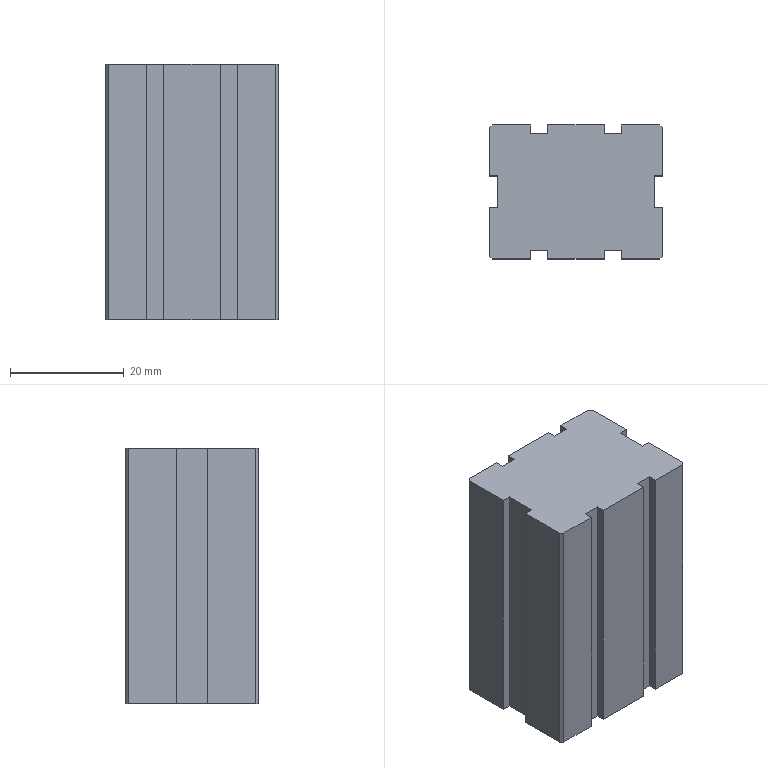Part | SolidWorks | features Extrusion 1 | 1 solid | 34 faces | box 30.5 x 23.5 x 45 mm | volume 30669 mm3 | plane 34
STEP:
#1=CARTESIAN_POINT('',(-8.,11.75,0.));
#2=VERTEX_POINT('',#1);
#3=CARTESIAN_POINT('',(-14.75,11.75,0.));
#4=VERTEX_POINT('',#3);
#5=CARTESIAN_POINT('',(-14.75,11.75,0.));
#6=DIRECTION('',(-1.,0.,0.));
#7=VECTOR('',#6,1000.);
#8=LINE('',#5,#7);
#9=EDGE_CURVE('',#2,#4,#8,.T.);
#10=ORIENTED_EDGE('',*,*,#9,.T.);
#11=CARTESIAN_POINT('',(-14.75,11.75,45.));
#12=VERTEX_POINT('',#11);
#13=CARTESIAN_POINT('',(-14.75,11.75,45.));
#14=DIRECTION('',(0.,0.,-1.));
#15=VECTOR('',#14,1000.);
#16=LINE('',#13,#15);
#17=EDGE_CURVE('',#12,#4,#16,.T.);
#18=ORIENTED_EDGE('',*,*,#17,.F.);
#19=CARTESIAN_POINT('',(-8.,11.75,45.));
#20=VERTEX_POINT('',#19);
#21=CARTESIAN_POINT('',(-14.75,11.75,45.));
#22=DIRECTION('',(-1.,0.,0.));
#23=VECTOR('',#22,1000.);
#24=LINE('',#21,#23);
#25=EDGE_CURVE('',#20,#12,#24,.T.);
#26=ORIENTED_EDGE('',*,*,#25,.F.);
#27=CARTESIAN_POINT('',(-8.,11.75,45.));
#28=DIRECTION('',(0.,0.,-1.));
#29=VECTOR('',#28,1000.);
#30=LINE('',#27,#29);
#31=EDGE_CURVE('',#20,#2,#30,.T.);
#32=ORIENTED_EDGE('',*,*,#31,.T.);
#33=EDGE_LOOP('',(#10,#18,#26,#32));
#34=FACE_OUTER_BOUND('',#33,.T.);
#35=CARTESIAN_POINT('',(-14.75,11.75,45.));
#36=DIRECTION('',(0.,-1.,0.));
#37=DIRECTION('',(1.,0.,0.));
#38=AXIS2_PLACEMENT_3D('',#35,#36,#37);
#39=PLANE('',#38);
#40=ADVANCED_FACE('',(#34),#39,.F.);
#41=CARTESIAN_POINT('',(-15.25,11.25,0.));
#42=VERTEX_POINT('',#41);
#43=CARTESIAN_POINT('',(-15.25,11.25,0.));
#44=DIRECTION('',(-0.7071,-0.7071,0.));
#45=VECTOR('',#44,1000.);
#46=LINE('',#43,#45);
#47=EDGE_CURVE('',#4,#42,#46,.T.);
#48=ORIENTED_EDGE('',*,*,#47,.T.);
#49=CARTESIAN_POINT('',(-15.25,11.25,45.));
#50=VERTEX_POINT('',#49);
#51=CARTESIAN_POINT('',(-15.25,11.25,45.));
#52=DIRECTION('',(0.,0.,-1.));
#53=VECTOR('',#52,1000.);
#54=LINE('',#51,#53);
#55=EDGE_CURVE('',#50,#42,#54,.T.);
#56=ORIENTED_EDGE('',*,*,#55,.F.);
#57=CARTESIAN_POINT('',(-15.25,11.25,45.));
#58=DIRECTION('',(-0.7071,-0.7071,0.));
#59=VECTOR('',#58,1000.);
#60=LINE('',#57,#59);
#61=EDGE_CURVE('',#12,#50,#60,.T.);
#62=ORIENTED_EDGE('',*,*,#61,.F.);
#63=ORIENTED_EDGE('',*,*,#17,.T.);
#64=EDGE_LOOP('',(#48,#56,#62,#63));
#65=FACE_OUTER_BOUND('',#64,.T.);
#66=CARTESIAN_POINT('',(-15.25,11.25,45.));
#67=DIRECTION('',(0.7071,-0.7071,0.));
#68=DIRECTION('',(0.7071,0.7071,0.));
#69=AXIS2_PLACEMENT_3D('',#66,#67,#68);
#70=PLANE('',#69);
#71=ADVANCED_FACE('',(#65),#70,.F.);
#72=CARTESIAN_POINT('',(-15.25,2.786,0.));
#73=VERTEX_POINT('',#72);
#74=CARTESIAN_POINT('',(-15.25,11.25,0.));
#75=DIRECTION('',(0.,-1.,0.));
#76=VECTOR('',#75,1000.);
#77=LINE('',#74,#76);
#78=EDGE_CURVE('',#42,#73,#77,.T.);
#79=ORIENTED_EDGE('',*,*,#78,.T.);
#80=CARTESIAN_POINT('',(-15.25,2.786,45.));
#81=VERTEX_POINT('',#80);
#82=CARTESIAN_POINT('',(-15.25,2.786,45.));
#83=DIRECTION('',(0.,0.,-1.));
#84=VECTOR('',#83,1000.);
#85=LINE('',#82,#84);
#86=EDGE_CURVE('',#81,#73,#85,.T.);
#87=ORIENTED_EDGE('',*,*,#86,.F.);
#88=CARTESIAN_POINT('',(-15.25,11.25,45.));
#89=DIRECTION('',(0.,-1.,0.));
#90=VECTOR('',#89,1000.);
#91=LINE('',#88,#90);
#92=EDGE_CURVE('',#50,#81,#91,.T.);
#93=ORIENTED_EDGE('',*,*,#92,.F.);
#94=ORIENTED_EDGE('',*,*,#55,.T.);
#95=EDGE_LOOP('',(#79,#87,#93,#94));
#96=FACE_OUTER_BOUND('',#95,.T.);
#97=CARTESIAN_POINT('',(-15.25,11.25,45.));
#98=DIRECTION('',(1.,0.,0.));
#99=DIRECTION('',(0.,0.,-1.));
#100=AXIS2_PLACEMENT_3D('',#97,#98,#99);
#101=PLANE('',#100);
#102=ADVANCED_FACE('',(#96),#101,.F.);
#103=CARTESIAN_POINT('',(-13.75,2.786,0.));
#104=VERTEX_POINT('',#103);
#105=CARTESIAN_POINT('',(-15.25,2.786,0.));
#106=DIRECTION('',(1.,0.,0.));
#107=VECTOR('',#106,1000.);
#108=LINE('',#105,#107);
#109=EDGE_CURVE('',#73,#104,#108,.T.);
#110=ORIENTED_EDGE('',*,*,#109,.T.);
#111=CARTESIAN_POINT('',(-13.75,2.786,45.));
#112=VERTEX_POINT('',#111);
#113=CARTESIAN_POINT('',(-13.75,2.786,45.));
#114=DIRECTION('',(0.,0.,-1.));
#115=VECTOR('',#114,1000.);
#116=LINE('',#113,#115);
#117=EDGE_CURVE('',#112,#104,#116,.T.);
#118=ORIENTED_EDGE('',*,*,#117,.F.);
#119=CARTESIAN_POINT('',(-15.25,2.786,45.));
#120=DIRECTION('',(1.,0.,0.));
#121=VECTOR('',#120,1000.);
#122=LINE('',#119,#121);
#123=EDGE_CURVE('',#81,#112,#122,.T.);
#124=ORIENTED_EDGE('',*,*,#123,.F.);
#125=ORIENTED_EDGE('',*,*,#86,.T.);
#126=EDGE_LOOP('',(#110,#118,#124,#125));
#127=FACE_OUTER_BOUND('',#126,.T.);
#128=CARTESIAN_POINT('',(-15.25,2.786,45.));
#129=DIRECTION('',(0.,1.,0.));
#130=DIRECTION('',(0.,0.,1.));
#131=AXIS2_PLACEMENT_3D('',#128,#129,#130);
#132=PLANE('',#131);
#133=ADVANCED_FACE('',(#127),#132,.F.);
#134=CARTESIAN_POINT('',(-13.75,-2.786,0.));
#135=VERTEX_POINT('',#134);
#136=CARTESIAN_POINT('',(-13.75,2.786,0.));
#137=DIRECTION('',(0.,-1.,0.));
#138=VECTOR('',#137,1000.);
#139=LINE('',#136,#138);
#140=EDGE_CURVE('',#104,#135,#139,.T.);
#141=ORIENTED_EDGE('',*,*,#140,.T.);
#142=CARTESIAN_POINT('',(-13.75,-2.786,45.));
#143=VERTEX_POINT('',#142);
#144=CARTESIAN_POINT('',(-13.75,-2.786,45.));
#145=DIRECTION('',(0.,0.,-1.));
#146=VECTOR('',#145,1000.);
#147=LINE('',#144,#146);
#148=EDGE_CURVE('',#143,#135,#147,.T.);
#149=ORIENTED_EDGE('',*,*,#148,.F.);
#150=CARTESIAN_POINT('',(-13.75,2.786,45.));
#151=DIRECTION('',(0.,-1.,0.));
#152=VECTOR('',#151,1000.);
#153=LINE('',#150,#152);
#154=EDGE_CURVE('',#112,#143,#153,.T.);
#155=ORIENTED_EDGE('',*,*,#154,.F.);
#156=ORIENTED_EDGE('',*,*,#117,.T.);
#157=EDGE_LOOP('',(#141,#149,#155,#156));
#158=FACE_OUTER_BOUND('',#157,.T.);
#159=CARTESIAN_POINT('',(-13.75,2.786,45.));
#160=DIRECTION('',(1.,0.,0.));
#161=DIRECTION('',(0.,0.,-1.));
#162=AXIS2_PLACEMENT_3D('',#159,#160,#161);
#163=PLANE('',#162);
#164=ADVANCED_FACE('',(#158),#163,.F.);
#165=CARTESIAN_POINT('',(-15.25,-2.786,0.));
#166=VERTEX_POINT('',#165);
#167=CARTESIAN_POINT('',(-15.25,-2.786,0.));
#168=DIRECTION('',(-1.,0.,0.));
#169=VECTOR('',#168,1000.);
#170=LINE('',#167,#169);
#171=EDGE_CURVE('',#135,#166,#170,.T.);
#172=ORIENTED_EDGE('',*,*,#171,.T.);
#173=CARTESIAN_POINT('',(-15.25,-2.786,45.));
#174=VERTEX_POINT('',#173);
#175=CARTESIAN_POINT('',(-15.25,-2.786,45.));
#176=DIRECTION('',(0.,0.,-1.));
#177=VECTOR('',#176,1000.);
#178=LINE('',#175,#177);
#179=EDGE_CURVE('',#174,#166,#178,.T.);
#180=ORIENTED_EDGE('',*,*,#179,.F.);
#181=CARTESIAN_POINT('',(-15.25,-2.786,45.));
#182=DIRECTION('',(-1.,0.,0.));
#183=VECTOR('',#182,1000.);
#184=LINE('',#181,#183);
#185=EDGE_CURVE('',#143,#174,#184,.T.);
#186=ORIENTED_EDGE('',*,*,#185,.F.);
#187=ORIENTED_EDGE('',*,*,#148,.T.);
#188=EDGE_LOOP('',(#172,#180,#186,#187));
#189=FACE_OUTER_BOUND('',#188,.T.);
#190=CARTESIAN_POINT('',(-15.25,-2.786,45.));
#191=DIRECTION('',(0.,-1.,0.));
#192=DIRECTION('',(0.,0.,-1.));
#193=AXIS2_PLACEMENT_3D('',#190,#191,#192);
#194=PLANE('',#193);
#195=ADVANCED_FACE('',(#189),#194,.F.);
#196=CARTESIAN_POINT('',(-15.25,-11.25,0.));
#197=VERTEX_POINT('',#196);
#198=CARTESIAN_POINT('',(-15.25,-2.786,0.));
#199=DIRECTION('',(0.,-1.,0.));
#200=VECTOR('',#199,1000.);
#201=LINE('',#198,#200);
#202=EDGE_CURVE('',#166,#197,#201,.T.);
#203=ORIENTED_EDGE('',*,*,#202,.T.);
#204=CARTESIAN_POINT('',(-15.25,-11.25,45.));
#205=VERTEX_POINT('',#204);
#206=CARTESIAN_POINT('',(-15.25,-11.25,45.));
#207=DIRECTION('',(0.,0.,-1.));
#208=VECTOR('',#207,1000.);
#209=LINE('',#206,#208);
#210=EDGE_CURVE('',#205,#197,#209,.T.);
#211=ORIENTED_EDGE('',*,*,#210,.F.);
#212=CARTESIAN_POINT('',(-15.25,-2.786,45.));
#213=DIRECTION('',(0.,-1.,0.));
#214=VECTOR('',#213,1000.);
#215=LINE('',#212,#214);
#216=EDGE_CURVE('',#174,#205,#215,.T.);
#217=ORIENTED_EDGE('',*,*,#216,.F.);
#218=ORIENTED_EDGE('',*,*,#179,.T.);
#219=EDGE_LOOP('',(#203,#211,#217,#218));
#220=FACE_OUTER_BOUND('',#219,.T.);
#221=CARTESIAN_POINT('',(-15.25,-2.786,45.));
#222=DIRECTION('',(1.,0.,0.));
#223=DIRECTION('',(0.,1.,0.));
#224=AXIS2_PLACEMENT_3D('',#221,#222,#223);
#225=PLANE('',#224);
#226=ADVANCED_FACE('',(#220),#225,.F.);
#227=CARTESIAN_POINT('',(-14.75,-11.75,0.));
#228=VERTEX_POINT('',#227);
#229=CARTESIAN_POINT('',(-15.25,-11.25,0.));
#230=DIRECTION('',(0.7071,-0.7071,0.));
#231=VECTOR('',#230,1000.);
#232=LINE('',#229,#231);
#233=EDGE_CURVE('',#197,#228,#232,.T.);
#234=ORIENTED_EDGE('',*,*,#233,.T.);
#235=CARTESIAN_POINT('',(-14.75,-11.75,45.));
#236=VERTEX_POINT('',#235);
#237=CARTESIAN_POINT('',(-14.75,-11.75,45.));
#238=DIRECTION('',(0.,0.,-1.));
#239=VECTOR('',#238,1000.);
#240=LINE('',#237,#239);
#241=EDGE_CURVE('',#236,#228,#240,.T.);
#242=ORIENTED_EDGE('',*,*,#241,.F.);
#243=CARTESIAN_POINT('',(-15.25,-11.25,45.));
#244=DIRECTION('',(0.7071,-0.7071,0.));
#245=VECTOR('',#244,1000.);
#246=LINE('',#243,#245);
#247=EDGE_CURVE('',#205,#236,#246,.T.);
#248=ORIENTED_EDGE('',*,*,#247,.F.);
#249=ORIENTED_EDGE('',*,*,#210,.T.);
#250=EDGE_LOOP('',(#234,#242,#248,#249));
#251=FACE_OUTER_BOUND('',#250,.T.);
#252=CARTESIAN_POINT('',(-15.25,-11.25,45.));
#253=DIRECTION('',(0.7071,0.7071,0.));
#254=DIRECTION('',(-0.7071,0.7071,0.));
#255=AXIS2_PLACEMENT_3D('',#252,#253,#254);
#256=PLANE('',#255);
#257=ADVANCED_FACE('',(#251),#256,.F.);
#258=CARTESIAN_POINT('',(-8.,-11.75,0.));
#259=VERTEX_POINT('',#258);
#260=CARTESIAN_POINT('',(-14.75,-11.75,0.));
#261=DIRECTION('',(1.,0.,0.));
#262=VECTOR('',#261,1000.);
#263=LINE('',#260,#262);
#264=EDGE_CURVE('',#228,#259,#263,.T.);
#265=ORIENTED_EDGE('',*,*,#264,.T.);
#266=CARTESIAN_POINT('',(-8.,-11.75,45.));
#267=VERTEX_POINT('',#266);
#268=CARTESIAN_POINT('',(-8.,-11.75,45.));
#269=DIRECTION('',(0.,0.,-1.));
#270=VECTOR('',#269,1000.);
#271=LINE('',#268,#270);
#272=EDGE_CURVE('',#267,#259,#271,.T.);
#273=ORIENTED_EDGE('',*,*,#272,.F.);
#274=CARTESIAN_POINT('',(-14.75,-11.75,45.));
#275=DIRECTION('',(1.,0.,0.));
#276=VECTOR('',#275,1000.);
#277=LINE('',#274,#276);
#278=EDGE_CURVE('',#236,#267,#277,.T.);
#279=ORIENTED_EDGE('',*,*,#278,.F.);
#280=ORIENTED_EDGE('',*,*,#241,.T.);
#281=EDGE_LOOP('',(#265,#273,#279,#280));
#282=FACE_OUTER_BOUND('',#281,.T.);
#283=CARTESIAN_POINT('',(-14.75,-11.75,45.));
#284=DIRECTION('',(0.,1.,0.));
#285=DIRECTION('',(0.,0.,1.));
#286=AXIS2_PLACEMENT_3D('',#283,#284,#285);
#287=PLANE('',#286);
#288=ADVANCED_FACE('',(#282),#287,.F.);
#289=CARTESIAN_POINT('',(-8.,-10.25,0.));
#290=VERTEX_POINT('',#289);
#291=CARTESIAN_POINT('',(-8.,-11.75,0.));
#292=DIRECTION('',(0.,1.,0.));
#293=VECTOR('',#292,1000.);
#294=LINE('',#291,#293);
#295=EDGE_CURVE('',#259,#290,#294,.T.);
#296=ORIENTED_EDGE('',*,*,#295,.T.);
#297=CARTESIAN_POINT('',(-8.,-10.25,45.));
#298=VERTEX_POINT('',#297);
#299=CARTESIAN_POINT('',(-8.,-10.25,45.));
#300=DIRECTION('',(0.,0.,-1.));
#301=VECTOR('',#300,1000.);
#302=LINE('',#299,#301);
#303=EDGE_CURVE('',#298,#290,#302,.T.);
#304=ORIENTED_EDGE('',*,*,#303,.F.);
#305=CARTESIAN_POINT('',(-8.,-11.75,45.));
#306=DIRECTION('',(0.,1.,0.));
#307=VECTOR('',#306,1000.);
#308=LINE('',#305,#307);
#309=EDGE_CURVE('',#267,#298,#308,.T.);
#310=ORIENTED_EDGE('',*,*,#309,.F.);
#311=ORIENTED_EDGE('',*,*,#272,.T.);
#312=EDGE_LOOP('',(#296,#304,#310,#311));
#313=FACE_OUTER_BOUND('',#312,.T.);
#314=CARTESIAN_POINT('',(-8.,-11.75,45.));
#315=DIRECTION('',(-1.,0.,0.));
#316=DIRECTION('',(0.,0.,1.));
#317=AXIS2_PLACEMENT_3D('',#314,#315,#316);
#318=PLANE('',#317);
#319=ADVANCED_FACE('',(#313),#318,.F.);
#320=CARTESIAN_POINT('',(-5.,-10.25,0.));
#321=VERTEX_POINT('',#320);
#322=CARTESIAN_POINT('',(-8.,-10.25,0.));
#323=DIRECTION('',(1.,0.,0.));
#324=VECTOR('',#323,1000.);
#325=LINE('',#322,#324);
#326=EDGE_CURVE('',#290,#321,#325,.T.);
#327=ORIENTED_EDGE('',*,*,#326,.T.);
#328=CARTESIAN_POINT('',(-5.,-10.25,45.));
#329=VERTEX_POINT('',#328);
#330=CARTESIAN_POINT('',(-5.,-10.25,45.));
#331=DIRECTION('',(0.,0.,-1.));
#332=VECTOR('',#331,1000.);
#333=LINE('',#330,#332);
#334=EDGE_CURVE('',#329,#321,#333,.T.);
#335=ORIENTED_EDGE('',*,*,#334,.F.);
#336=CARTESIAN_POINT('',(-8.,-10.25,45.));
#337=DIRECTION('',(1.,0.,0.));
#338=VECTOR('',#337,1000.);
#339=LINE('',#336,#338);
#340=EDGE_CURVE('',#298,#329,#339,.T.);
#341=ORIENTED_EDGE('',*,*,#340,.F.);
#342=ORIENTED_EDGE('',*,*,#303,.T.);
#343=EDGE_LOOP('',(#327,#335,#341,#342));
#344=FACE_OUTER_BOUND('',#343,.T.);
#345=CARTESIAN_POINT('',(-8.,-10.25,45.));
#346=DIRECTION('',(0.,1.,0.));
#347=DIRECTION('',(0.,0.,1.));
#348=AXIS2_PLACEMENT_3D('',#345,#346,#347);
#349=PLANE('',#348);
#350=ADVANCED_FACE('',(#344),#349,.F.);
#351=CARTESIAN_POINT('',(-5.,-11.75,0.));
#352=VERTEX_POINT('',#351);
#353=CARTESIAN_POINT('',(-5.,-10.25,0.));
#354=DIRECTION('',(0.,-1.,0.));
#355=VECTOR('',#354,1000.);
#356=LINE('',#353,#355);
#357=EDGE_CURVE('',#321,#352,#356,.T.);
#358=ORIENTED_EDGE('',*,*,#357,.T.);
#359=CARTESIAN_POINT('',(-5.,-11.75,45.));
#360=VERTEX_POINT('',#359);
#361=CARTESIAN_POINT('',(-5.,-11.75,45.));
#362=DIRECTION('',(0.,0.,-1.));
#363=VECTOR('',#362,1000.);
#364=LINE('',#361,#363);
#365=EDGE_CURVE('',#360,#352,#364,.T.);
#366=ORIENTED_EDGE('',*,*,#365,.F.);
#367=CARTESIAN_POINT('',(-5.,-10.25,45.));
#368=DIRECTION('',(0.,-1.,0.));
#369=VECTOR('',#368,1000.);
#370=LINE('',#367,#369);
#371=EDGE_CURVE('',#329,#360,#370,.T.);
#372=ORIENTED_EDGE('',*,*,#371,.F.);
#373=ORIENTED_EDGE('',*,*,#334,.T.);
#374=EDGE_LOOP('',(#358,#366,#372,#373));
#375=FACE_OUTER_BOUND('',#374,.T.);
#376=CARTESIAN_POINT('',(-5.,-10.25,45.));
#377=DIRECTION('',(1.,0.,0.));
#378=DIRECTION('',(0.,0.,-1.));
#379=AXIS2_PLACEMENT_3D('',#376,#377,#378);
#380=PLANE('',#379);
#381=ADVANCED_FACE('',(#375),#380,.F.);
#382=CARTESIAN_POINT('',(5.,-11.75,0.));
#383=VERTEX_POINT('',#382);
#384=CARTESIAN_POINT('',(-5.,-11.75,0.));
#385=DIRECTION('',(1.,0.,0.));
#386=VECTOR('',#385,1000.);
#387=LINE('',#384,#386);
#388=EDGE_CURVE('',#352,#383,#387,.T.);
#389=ORIENTED_EDGE('',*,*,#388,.T.);
#390=CARTESIAN_POINT('',(5.,-11.75,45.));
#391=VERTEX_POINT('',#390);
#392=CARTESIAN_POINT('',(5.,-11.75,45.));
#393=DIRECTION('',(0.,0.,-1.));
#394=VECTOR('',#393,1000.);
#395=LINE('',#392,#394);
#396=EDGE_CURVE('',#391,#383,#395,.T.);
#397=ORIENTED_EDGE('',*,*,#396,.F.);
#398=CARTESIAN_POINT('',(-5.,-11.75,45.));
#399=DIRECTION('',(1.,0.,0.));
#400=VECTOR('',#399,1000.);
#401=LINE('',#398,#400);
#402=EDGE_CURVE('',#360,#391,#401,.T.);
#403=ORIENTED_EDGE('',*,*,#402,.F.);
#404=ORIENTED_EDGE('',*,*,#365,.T.);
#405=EDGE_LOOP('',(#389,#397,#403,#404));
#406=FACE_OUTER_BOUND('',#405,.T.);
#407=CARTESIAN_POINT('',(-5.,-11.75,45.));
#408=DIRECTION('',(0.,1.,0.));
#409=DIRECTION('',(0.,0.,1.));
#410=AXIS2_PLACEMENT_3D('',#407,#408,#409);
#411=PLANE('',#410);
#412=ADVANCED_FACE('',(#406),#411,.F.);
#413=CARTESIAN_POINT('',(5.,-10.25,0.));
#414=VERTEX_POINT('',#413);
#415=CARTESIAN_POINT('',(5.,-10.25,0.));
#416=DIRECTION('',(0.,1.,0.));
#417=VECTOR('',#416,1000.);
#418=LINE('',#415,#417);
#419=EDGE_CURVE('',#383,#414,#418,.T.);
#420=ORIENTED_EDGE('',*,*,#419,.T.);
#421=CARTESIAN_POINT('',(5.,-10.25,45.));
#422=VERTEX_POINT('',#421);
#423=CARTESIAN_POINT('',(5.,-10.25,45.));
#424=DIRECTION('',(0.,0.,-1.));
#425=VECTOR('',#424,1000.);
#426=LINE('',#423,#425);
#427=EDGE_CURVE('',#422,#414,#426,.T.);
#428=ORIENTED_EDGE('',*,*,#427,.F.);
#429=CARTESIAN_POINT('',(5.,-10.25,45.));
#430=DIRECTION('',(0.,1.,0.));
#431=VECTOR('',#430,1000.);
#432=LINE('',#429,#431);
#433=EDGE_CURVE('',#391,#422,#432,.T.);
#434=ORIENTED_EDGE('',*,*,#433,.F.);
#435=ORIENTED_EDGE('',*,*,#396,.T.);
#436=EDGE_LOOP('',(#420,#428,#434,#435));
#437=FACE_OUTER_BOUND('',#436,.T.);
#438=CARTESIAN_POINT('',(5.,-10.25,45.));
#439=DIRECTION('',(-1.,0.,0.));
#440=DIRECTION('',(0.,0.,1.));
#441=AXIS2_PLACEMENT_3D('',#438,#439,#440);
#442=PLANE('',#441);
#443=ADVANCED_FACE('',(#437),#442,.F.);
#444=CARTESIAN_POINT('',(8.,-10.25,0.));
#445=VERTEX_POINT('',#444);
#446=CARTESIAN_POINT('',(8.,-10.25,0.));
#447=DIRECTION('',(1.,0.,0.));
#448=VECTOR('',#447,1000.);
#449=LINE('',#446,#448);
#450=EDGE_CURVE('',#414,#445,#449,.T.);
#451=ORIENTED_EDGE('',*,*,#450,.T.);
#452=CARTESIAN_POINT('',(8.,-10.25,45.));
#453=VERTEX_POINT('',#452);
#454=CARTESIAN_POINT('',(8.,-10.25,45.));
#455=DIRECTION('',(0.,0.,-1.));
#456=VECTOR('',#455,1000.);
#457=LINE('',#454,#456);
#458=EDGE_CURVE('',#453,#445,#457,.T.);
#459=ORIENTED_EDGE('',*,*,#458,.F.);
#460=CARTESIAN_POINT('',(8.,-10.25,45.));
#461=DIRECTION('',(1.,0.,0.));
#462=VECTOR('',#461,1000.);
#463=LINE('',#460,#462);
#464=EDGE_CURVE('',#422,#453,#463,.T.);
#465=ORIENTED_EDGE('',*,*,#464,.F.);
#466=ORIENTED_EDGE('',*,*,#427,.T.);
#467=EDGE_LOOP('',(#451,#459,#465,#466));
#468=FACE_OUTER_BOUND('',#467,.T.);
#469=CARTESIAN_POINT('',(8.,-10.25,45.));
#470=DIRECTION('',(0.,1.,0.));
#471=DIRECTION('',(0.,0.,1.));
#472=AXIS2_PLACEMENT_3D('',#469,#470,#471);
#473=PLANE('',#472);
#474=ADVANCED_FACE('',(#468),#473,.F.);
#475=CARTESIAN_POINT('',(8.,-11.75,0.));
#476=VERTEX_POINT('',#475);
#477=CARTESIAN_POINT('',(8.,-11.75,0.));
#478=DIRECTION('',(0.,-1.,0.));
#479=VECTOR('',#478,1000.);
#480=LINE('',#477,#479);
#481=EDGE_CURVE('',#445,#476,#480,.T.);
#482=ORIENTED_EDGE('',*,*,#481,.T.);
#483=CARTESIAN_POINT('',(8.,-11.75,45.));
#484=VERTEX_POINT('',#483);
#485=CARTESIAN_POINT('',(8.,-11.75,45.));
#486=DIRECTION('',(0.,0.,-1.));
#487=VECTOR('',#486,1000.);
#488=LINE('',#485,#487);
#489=EDGE_CURVE('',#484,#476,#488,.T.);
#490=ORIENTED_EDGE('',*,*,#489,.F.);
#491=CARTESIAN_POINT('',(8.,-11.75,45.));
#492=DIRECTION('',(0.,-1.,0.));
#493=VECTOR('',#492,1000.);
#494=LINE('',#491,#493);
#495=EDGE_CURVE('',#453,#484,#494,.T.);
#496=ORIENTED_EDGE('',*,*,#495,.F.);
#497=ORIENTED_EDGE('',*,*,#458,.T.);
#498=EDGE_LOOP('',(#482,#490,#496,#497));
#499=FACE_OUTER_BOUND('',#498,.T.);
#500=CARTESIAN_POINT('',(8.,-11.75,45.));
#501=DIRECTION('',(1.,0.,0.));
#502=DIRECTION('',(0.,0.,-1.));
#503=AXIS2_PLACEMENT_3D('',#500,#501,#502);
#504=PLANE('',#503);
#505=ADVANCED_FACE('',(#499),#504,.F.);
#506=CARTESIAN_POINT('',(14.75,-11.75,0.));
#507=VERTEX_POINT('',#506);
#508=CARTESIAN_POINT('',(8.,-11.75,0.));
#509=DIRECTION('',(1.,0.,0.));
#510=VECTOR('',#509,1000.);
#511=LINE('',#508,#510);
#512=EDGE_CURVE('',#476,#507,#511,.T.);
#513=ORIENTED_EDGE('',*,*,#512,.T.);
#514=CARTESIAN_POINT('',(14.75,-11.75,45.));
#515=VERTEX_POINT('',#514);
#516=CARTESIAN_POINT('',(14.75,-11.75,45.));
#517=DIRECTION('',(0.,0.,-1.));
#518=VECTOR('',#517,1000.);
#519=LINE('',#516,#518);
#520=EDGE_CURVE('',#515,#507,#519,.T.);
#521=ORIENTED_EDGE('',*,*,#520,.F.);
#522=CARTESIAN_POINT('',(8.,-11.75,45.));
#523=DIRECTION('',(1.,0.,0.));
#524=VECTOR('',#523,1000.);
#525=LINE('',#522,#524);
#526=EDGE_CURVE('',#484,#515,#525,.T.);
#527=ORIENTED_EDGE('',*,*,#526,.F.);
#528=ORIENTED_EDGE('',*,*,#489,.T.);
#529=EDGE_LOOP('',(#513,#521,#527,#528));
#530=FACE_OUTER_BOUND('',#529,.T.);
#531=CARTESIAN_POINT('',(8.,-11.75,45.));
#532=DIRECTION('',(0.,1.,0.));
#533=DIRECTION('',(0.,0.,1.));
#534=AXIS2_PLACEMENT_3D('',#531,#532,#533);
#535=PLANE('',#534);
#536=ADVANCED_FACE('',(#530),#535,.F.);
#537=CARTESIAN_POINT('',(15.25,-11.25,0.));
#538=VERTEX_POINT('',#537);
#539=CARTESIAN_POINT('',(14.75,-11.75,0.));
#540=DIRECTION('',(0.7071,0.7071,0.));
#541=VECTOR('',#540,1000.);
#542=LINE('',#539,#541);
#543=EDGE_CURVE('',#507,#538,#542,.T.);
#544=ORIENTED_EDGE('',*,*,#543,.T.);
#545=CARTESIAN_POINT('',(15.25,-11.25,45.));
#546=VERTEX_POINT('',#545);
#547=CARTESIAN_POINT('',(15.25,-11.25,45.));
#548=DIRECTION('',(0.,0.,-1.));
#549=VECTOR('',#548,1000.);
#550=LINE('',#547,#549);
#551=EDGE_CURVE('',#546,#538,#550,.T.);
#552=ORIENTED_EDGE('',*,*,#551,.F.);
#553=CARTESIAN_POINT('',(14.75,-11.75,45.));
#554=DIRECTION('',(0.7071,0.7071,0.));
#555=VECTOR('',#554,1000.);
#556=LINE('',#553,#555);
#557=EDGE_CURVE('',#515,#546,#556,.T.);
#558=ORIENTED_EDGE('',*,*,#557,.F.);
#559=ORIENTED_EDGE('',*,*,#520,.T.);
#560=EDGE_LOOP('',(#544,#552,#558,#559));
#561=FACE_OUTER_BOUND('',#560,.T.);
#562=CARTESIAN_POINT('',(14.75,-11.75,45.));
#563=DIRECTION('',(-0.7071,0.7071,0.));
#564=DIRECTION('',(-0.7071,-0.7071,0.));
#565=AXIS2_PLACEMENT_3D('',#562,#563,#564);
#566=PLANE('',#565);
#567=ADVANCED_FACE('',(#561),#566,.F.);
#568=CARTESIAN_POINT('',(15.25,-2.786,0.));
#569=VERTEX_POINT('',#568);
#570=CARTESIAN_POINT('',(15.25,-2.786,0.));
#571=DIRECTION('',(0.,1.,0.));
#572=VECTOR('',#571,1000.);
#573=LINE('',#570,#572);
#574=EDGE_CURVE('',#538,#569,#573,.T.);
#575=ORIENTED_EDGE('',*,*,#574,.T.);
#576=CARTESIAN_POINT('',(15.25,-2.786,45.));
#577=VERTEX_POINT('',#576);
#578=CARTESIAN_POINT('',(15.25,-2.786,45.));
#579=DIRECTION('',(0.,0.,-1.));
#580=VECTOR('',#579,1000.);
#581=LINE('',#578,#580);
#582=EDGE_CURVE('',#577,#569,#581,.T.);
#583=ORIENTED_EDGE('',*,*,#582,.F.);
#584=CARTESIAN_POINT('',(15.25,-2.786,45.));
#585=DIRECTION('',(0.,1.,0.));
#586=VECTOR('',#585,1000.);
#587=LINE('',#584,#586);
#588=EDGE_CURVE('',#546,#577,#587,.T.);
#589=ORIENTED_EDGE('',*,*,#588,.F.);
#590=ORIENTED_EDGE('',*,*,#551,.T.);
#591=EDGE_LOOP('',(#575,#583,#589,#590));
#592=FACE_OUTER_BOUND('',#591,.T.);
#593=CARTESIAN_POINT('',(15.25,-2.786,45.));
#594=DIRECTION('',(-1.,0.,0.));
#595=DIRECTION('',(0.,-1.,0.));
#596=AXIS2_PLACEMENT_3D('',#593,#594,#595);
#597=PLANE('',#596);
#598=ADVANCED_FACE('',(#592),#597,.F.);
#599=CARTESIAN_POINT('',(13.75,-2.786,0.));
#600=VERTEX_POINT('',#599);
#601=CARTESIAN_POINT('',(15.25,-2.786,0.));
#602=DIRECTION('',(-1.,0.,0.));
#603=VECTOR('',#602,1000.);
#604=LINE('',#601,#603);
#605=EDGE_CURVE('',#569,#600,#604,.T.);
#606=ORIENTED_EDGE('',*,*,#605,.T.);
#607=CARTESIAN_POINT('',(13.75,-2.786,45.));
#608=VERTEX_POINT('',#607);
#609=CARTESIAN_POINT('',(13.75,-2.786,45.));
#610=DIRECTION('',(0.,0.,-1.));
#611=VECTOR('',#610,1000.);
#612=LINE('',#609,#611);
#613=EDGE_CURVE('',#608,#600,#612,.T.);
#614=ORIENTED_EDGE('',*,*,#613,.F.);
#615=CARTESIAN_POINT('',(15.25,-2.786,45.));
#616=DIRECTION('',(-1.,0.,0.));
#617=VECTOR('',#616,1000.);
#618=LINE('',#615,#617);
#619=EDGE_CURVE('',#577,#608,#618,.T.);
#620=ORIENTED_EDGE('',*,*,#619,.F.);
#621=ORIENTED_EDGE('',*,*,#582,.T.);
#622=EDGE_LOOP('',(#606,#614,#620,#621));
#623=FACE_OUTER_BOUND('',#622,.T.);
#624=CARTESIAN_POINT('',(15.25,-2.786,45.));
#625=DIRECTION('',(0.,-1.,0.));
#626=DIRECTION('',(0.,0.,-1.));
#627=AXIS2_PLACEMENT_3D('',#624,#625,#626);
#628=PLANE('',#627);
#629=ADVANCED_FACE('',(#623),#628,.F.);
#630=CARTESIAN_POINT('',(13.75,2.786,0.));
#631=VERTEX_POINT('',#630);
#632=CARTESIAN_POINT('',(13.75,2.786,0.));
#633=DIRECTION('',(0.,1.,0.));
#634=VECTOR('',#633,1000.);
#635=LINE('',#632,#634);
#636=EDGE_CURVE('',#600,#631,#635,.T.);
#637=ORIENTED_EDGE('',*,*,#636,.T.);
#638=CARTESIAN_POINT('',(13.75,2.786,45.));
#639=VERTEX_POINT('',#638);
#640=CARTESIAN_POINT('',(13.75,2.786,45.));
#641=DIRECTION('',(0.,0.,-1.));
#642=VECTOR('',#641,1000.);
#643=LINE('',#640,#642);
#644=EDGE_CURVE('',#639,#631,#643,.T.);
#645=ORIENTED_EDGE('',*,*,#644,.F.);
#646=CARTESIAN_POINT('',(13.75,2.786,45.));
#647=DIRECTION('',(0.,1.,0.));
#648=VECTOR('',#647,1000.);
#649=LINE('',#646,#648);
#650=EDGE_CURVE('',#608,#639,#649,.T.);
#651=ORIENTED_EDGE('',*,*,#650,.F.);
#652=ORIENTED_EDGE('',*,*,#613,.T.);
#653=EDGE_LOOP('',(#637,#645,#651,#652));
#654=FACE_OUTER_BOUND('',#653,.T.);
#655=CARTESIAN_POINT('',(13.75,2.786,45.));
#656=DIRECTION('',(-1.,0.,0.));
#657=DIRECTION('',(0.,0.,1.));
#658=AXIS2_PLACEMENT_3D('',#655,#656,#657);
#659=PLANE('',#658);
#660=ADVANCED_FACE('',(#654),#659,.F.);
#661=CARTESIAN_POINT('',(15.25,2.786,0.));
#662=VERTEX_POINT('',#661);
#663=CARTESIAN_POINT('',(15.25,2.786,0.));
#664=DIRECTION('',(1.,0.,0.));
#665=VECTOR('',#664,1000.);
#666=LINE('',#663,#665);
#667=EDGE_CURVE('',#631,#662,#666,.T.);
#668=ORIENTED_EDGE('',*,*,#667,.T.);
#669=CARTESIAN_POINT('',(15.25,2.786,45.));
#670=VERTEX_POINT('',#669);
#671=CARTESIAN_POINT('',(15.25,2.786,45.));
#672=DIRECTION('',(0.,0.,-1.));
#673=VECTOR('',#672,1000.);
#674=LINE('',#671,#673);
#675=EDGE_CURVE('',#670,#662,#674,.T.);
#676=ORIENTED_EDGE('',*,*,#675,.F.);
#677=CARTESIAN_POINT('',(15.25,2.786,45.));
#678=DIRECTION('',(1.,0.,0.));
#679=VECTOR('',#678,1000.);
#680=LINE('',#677,#679);
#681=EDGE_CURVE('',#639,#670,#680,.T.);
#682=ORIENTED_EDGE('',*,*,#681,.F.);
#683=ORIENTED_EDGE('',*,*,#644,.T.);
#684=EDGE_LOOP('',(#668,#676,#682,#683));
#685=FACE_OUTER_BOUND('',#684,.T.);
#686=CARTESIAN_POINT('',(15.25,2.786,45.));
#687=DIRECTION('',(0.,1.,0.));
#688=DIRECTION('',(0.,0.,1.));
#689=AXIS2_PLACEMENT_3D('',#686,#687,#688);
#690=PLANE('',#689);
#691=ADVANCED_FACE('',(#685),#690,.F.);
#692=CARTESIAN_POINT('',(15.25,11.25,0.));
#693=VERTEX_POINT('',#692);
#694=CARTESIAN_POINT('',(15.25,11.25,0.));
#695=DIRECTION('',(0.,1.,0.));
#696=VECTOR('',#695,1000.);
#697=LINE('',#694,#696);
#698=EDGE_CURVE('',#662,#693,#697,.T.);
#699=ORIENTED_EDGE('',*,*,#698,.T.);
#700=CARTESIAN_POINT('',(15.25,11.25,45.));
#701=VERTEX_POINT('',#700);
#702=CARTESIAN_POINT('',(15.25,11.25,45.));
#703=DIRECTION('',(0.,0.,-1.));
#704=VECTOR('',#703,1000.);
#705=LINE('',#702,#704);
#706=EDGE_CURVE('',#701,#693,#705,.T.);
#707=ORIENTED_EDGE('',*,*,#706,.F.);
#708=CARTESIAN_POINT('',(15.25,11.25,45.));
#709=DIRECTION('',(0.,1.,0.));
#710=VECTOR('',#709,1000.);
#711=LINE('',#708,#710);
#712=EDGE_CURVE('',#670,#701,#711,.T.);
#713=ORIENTED_EDGE('',*,*,#712,.F.);
#714=ORIENTED_EDGE('',*,*,#675,.T.);
#715=EDGE_LOOP('',(#699,#707,#713,#714));
#716=FACE_OUTER_BOUND('',#715,.T.);
#717=CARTESIAN_POINT('',(15.25,11.25,45.));
#718=DIRECTION('',(-1.,0.,0.));
#719=DIRECTION('',(0.,0.,1.));
#720=AXIS2_PLACEMENT_3D('',#717,#718,#719);
#721=PLANE('',#720);
#722=ADVANCED_FACE('',(#716),#721,.F.);
#723=CARTESIAN_POINT('',(14.75,11.75,0.));
#724=VERTEX_POINT('',#723);
#725=CARTESIAN_POINT('',(14.75,11.75,0.));
#726=DIRECTION('',(-0.7071,0.7071,0.));
#727=VECTOR('',#726,1000.);
#728=LINE('',#725,#727);
#729=EDGE_CURVE('',#693,#724,#728,.T.);
#730=ORIENTED_EDGE('',*,*,#729,.T.);
#731=CARTESIAN_POINT('',(14.75,11.75,45.));
#732=VERTEX_POINT('',#731);
#733=CARTESIAN_POINT('',(14.75,11.75,45.));
#734=DIRECTION('',(0.,0.,-1.));
#735=VECTOR('',#734,1000.);
#736=LINE('',#733,#735);
#737=EDGE_CURVE('',#732,#724,#736,.T.);
#738=ORIENTED_EDGE('',*,*,#737,.F.);
#739=CARTESIAN_POINT('',(14.75,11.75,45.));
#740=DIRECTION('',(-0.7071,0.7071,0.));
#741=VECTOR('',#740,1000.);
#742=LINE('',#739,#741);
#743=EDGE_CURVE('',#701,#732,#742,.T.);
#744=ORIENTED_EDGE('',*,*,#743,.F.);
#745=ORIENTED_EDGE('',*,*,#706,.T.);
#746=EDGE_LOOP('',(#730,#738,#744,#745));
#747=FACE_OUTER_BOUND('',#746,.T.);
#748=CARTESIAN_POINT('',(14.75,11.75,45.));
#749=DIRECTION('',(-0.7071,-0.7071,0.));
#750=DIRECTION('',(0.7071,-0.7071,0.));
#751=AXIS2_PLACEMENT_3D('',#748,#749,#750);
#752=PLANE('',#751);
#753=ADVANCED_FACE('',(#747),#752,.F.);
#754=CARTESIAN_POINT('',(8.,11.75,0.));
#755=VERTEX_POINT('',#754);
#756=CARTESIAN_POINT('',(8.,11.75,0.));
#757=DIRECTION('',(-1.,0.,0.));
#758=VECTOR('',#757,1000.);
#759=LINE('',#756,#758);
#760=EDGE_CURVE('',#724,#755,#759,.T.);
#761=ORIENTED_EDGE('',*,*,#760,.T.);
#762=CARTESIAN_POINT('',(8.,11.75,45.));
#763=VERTEX_POINT('',#762);
#764=CARTESIAN_POINT('',(8.,11.75,45.));
#765=DIRECTION('',(0.,0.,-1.));
#766=VECTOR('',#765,1000.);
#767=LINE('',#764,#766);
#768=EDGE_CURVE('',#763,#755,#767,.T.);
#769=ORIENTED_EDGE('',*,*,#768,.F.);
#770=CARTESIAN_POINT('',(8.,11.75,45.));
#771=DIRECTION('',(-1.,0.,0.));
#772=VECTOR('',#771,1000.);
#773=LINE('',#770,#772);
#774=EDGE_CURVE('',#732,#763,#773,.T.);
#775=ORIENTED_EDGE('',*,*,#774,.F.);
#776=ORIENTED_EDGE('',*,*,#737,.T.);
#777=EDGE_LOOP('',(#761,#769,#775,#776));
#778=FACE_OUTER_BOUND('',#777,.T.);
#779=CARTESIAN_POINT('',(8.,11.75,45.));
#780=DIRECTION('',(0.,-1.,0.));
#781=DIRECTION('',(1.,0.,0.));
#782=AXIS2_PLACEMENT_3D('',#779,#780,#781);
#783=PLANE('',#782);
#784=ADVANCED_FACE('',(#778),#783,.F.);
#785=CARTESIAN_POINT('',(8.,10.25,0.));
#786=VERTEX_POINT('',#785);
#787=CARTESIAN_POINT('',(8.,11.75,0.));
#788=DIRECTION('',(0.,-1.,0.));
#789=VECTOR('',#788,1000.);
#790=LINE('',#787,#789);
#791=EDGE_CURVE('',#755,#786,#790,.T.);
#792=ORIENTED_EDGE('',*,*,#791,.T.);
#793=CARTESIAN_POINT('',(8.,10.25,45.));
#794=VERTEX_POINT('',#793);
#795=CARTESIAN_POINT('',(8.,10.25,45.));
#796=DIRECTION('',(0.,0.,-1.));
#797=VECTOR('',#796,1000.);
#798=LINE('',#795,#797);
#799=EDGE_CURVE('',#794,#786,#798,.T.);
#800=ORIENTED_EDGE('',*,*,#799,.F.);
#801=CARTESIAN_POINT('',(8.,11.75,45.));
#802=DIRECTION('',(0.,-1.,0.));
#803=VECTOR('',#802,1000.);
#804=LINE('',#801,#803);
#805=EDGE_CURVE('',#763,#794,#804,.T.);
#806=ORIENTED_EDGE('',*,*,#805,.F.);
#807=ORIENTED_EDGE('',*,*,#768,.T.);
#808=EDGE_LOOP('',(#792,#800,#806,#807));
#809=FACE_OUTER_BOUND('',#808,.T.);
#810=CARTESIAN_POINT('',(8.,11.75,45.));
#811=DIRECTION('',(1.,0.,0.));
#812=DIRECTION('',(0.,0.,-1.));
#813=AXIS2_PLACEMENT_3D('',#810,#811,#812);
#814=PLANE('',#813);
#815=ADVANCED_FACE('',(#809),#814,.F.);
#816=CARTESIAN_POINT('',(5.,10.25,0.));
#817=VERTEX_POINT('',#816);
#818=CARTESIAN_POINT('',(8.,10.25,0.));
#819=DIRECTION('',(-1.,0.,0.));
#820=VECTOR('',#819,1000.);
#821=LINE('',#818,#820);
#822=EDGE_CURVE('',#786,#817,#821,.T.);
#823=ORIENTED_EDGE('',*,*,#822,.T.);
#824=CARTESIAN_POINT('',(5.,10.25,45.));
#825=VERTEX_POINT('',#824);
#826=CARTESIAN_POINT('',(5.,10.25,45.));
#827=DIRECTION('',(0.,0.,-1.));
#828=VECTOR('',#827,1000.);
#829=LINE('',#826,#828);
#830=EDGE_CURVE('',#825,#817,#829,.T.);
#831=ORIENTED_EDGE('',*,*,#830,.F.);
#832=CARTESIAN_POINT('',(8.,10.25,45.));
#833=DIRECTION('',(-1.,0.,0.));
#834=VECTOR('',#833,1000.);
#835=LINE('',#832,#834);
#836=EDGE_CURVE('',#794,#825,#835,.T.);
#837=ORIENTED_EDGE('',*,*,#836,.F.);
#838=ORIENTED_EDGE('',*,*,#799,.T.);
#839=EDGE_LOOP('',(#823,#831,#837,#838));
#840=FACE_OUTER_BOUND('',#839,.T.);
#841=CARTESIAN_POINT('',(8.,10.25,45.));
#842=DIRECTION('',(0.,-1.,0.));
#843=DIRECTION('',(0.,0.,-1.));
#844=AXIS2_PLACEMENT_3D('',#841,#842,#843);
#845=PLANE('',#844);
#846=ADVANCED_FACE('',(#840),#845,.F.);
#847=CARTESIAN_POINT('',(5.,11.75,0.));
#848=VERTEX_POINT('',#847);
#849=CARTESIAN_POINT('',(5.,10.25,0.));
#850=DIRECTION('',(0.,1.,0.));
#851=VECTOR('',#850,1000.);
#852=LINE('',#849,#851);
#853=EDGE_CURVE('',#817,#848,#852,.T.);
#854=ORIENTED_EDGE('',*,*,#853,.T.);
#855=CARTESIAN_POINT('',(5.,11.75,45.));
#856=VERTEX_POINT('',#855);
#857=CARTESIAN_POINT('',(5.,11.75,45.));
#858=DIRECTION('',(0.,0.,-1.));
#859=VECTOR('',#858,1000.);
#860=LINE('',#857,#859);
#861=EDGE_CURVE('',#856,#848,#860,.T.);
#862=ORIENTED_EDGE('',*,*,#861,.F.);
#863=CARTESIAN_POINT('',(5.,10.25,45.));
#864=DIRECTION('',(0.,1.,0.));
#865=VECTOR('',#864,1000.);
#866=LINE('',#863,#865);
#867=EDGE_CURVE('',#825,#856,#866,.T.);
#868=ORIENTED_EDGE('',*,*,#867,.F.);
#869=ORIENTED_EDGE('',*,*,#830,.T.);
#870=EDGE_LOOP('',(#854,#862,#868,#869));
#871=FACE_OUTER_BOUND('',#870,.T.);
#872=CARTESIAN_POINT('',(5.,10.25,45.));
#873=DIRECTION('',(-1.,0.,0.));
#874=DIRECTION('',(0.,0.,1.));
#875=AXIS2_PLACEMENT_3D('',#872,#873,#874);
#876=PLANE('',#875);
#877=ADVANCED_FACE('',(#871),#876,.F.);
#878=CARTESIAN_POINT('',(-5.,11.75,0.));
#879=VERTEX_POINT('',#878);
#880=CARTESIAN_POINT('',(-5.,11.75,0.));
#881=DIRECTION('',(-1.,0.,0.));
#882=VECTOR('',#881,1000.);
#883=LINE('',#880,#882);
#884=EDGE_CURVE('',#848,#879,#883,.T.);
#885=ORIENTED_EDGE('',*,*,#884,.T.);
#886=CARTESIAN_POINT('',(-5.,11.75,45.));
#887=VERTEX_POINT('',#886);
#888=CARTESIAN_POINT('',(-5.,11.75,45.));
#889=DIRECTION('',(0.,0.,-1.));
#890=VECTOR('',#889,1000.);
#891=LINE('',#888,#890);
#892=EDGE_CURVE('',#887,#879,#891,.T.);
#893=ORIENTED_EDGE('',*,*,#892,.F.);
#894=CARTESIAN_POINT('',(-5.,11.75,45.));
#895=DIRECTION('',(-1.,0.,0.));
#896=VECTOR('',#895,1000.);
#897=LINE('',#894,#896);
#898=EDGE_CURVE('',#856,#887,#897,.T.);
#899=ORIENTED_EDGE('',*,*,#898,.F.);
#900=ORIENTED_EDGE('',*,*,#861,.T.);
#901=EDGE_LOOP('',(#885,#893,#899,#900));
#902=FACE_OUTER_BOUND('',#901,.T.);
#903=CARTESIAN_POINT('',(-5.,11.75,45.));
#904=DIRECTION('',(0.,-1.,0.));
#905=DIRECTION('',(0.,0.,-1.));
#906=AXIS2_PLACEMENT_3D('',#903,#904,#905);
#907=PLANE('',#906);
#908=ADVANCED_FACE('',(#902),#907,.F.);
#909=CARTESIAN_POINT('',(-5.,10.25,0.));
#910=VERTEX_POINT('',#909);
#911=CARTESIAN_POINT('',(-5.,10.25,0.));
#912=DIRECTION('',(0.,-1.,0.));
#913=VECTOR('',#912,1000.);
#914=LINE('',#911,#913);
#915=EDGE_CURVE('',#879,#910,#914,.T.);
#916=ORIENTED_EDGE('',*,*,#915,.T.);
#917=CARTESIAN_POINT('',(-5.,10.25,45.));
#918=VERTEX_POINT('',#917);
#919=CARTESIAN_POINT('',(-5.,10.25,45.));
#920=DIRECTION('',(0.,0.,-1.));
#921=VECTOR('',#920,1000.);
#922=LINE('',#919,#921);
#923=EDGE_CURVE('',#918,#910,#922,.T.);
#924=ORIENTED_EDGE('',*,*,#923,.F.);
#925=CARTESIAN_POINT('',(-5.,10.25,45.));
#926=DIRECTION('',(0.,-1.,0.));
#927=VECTOR('',#926,1000.);
#928=LINE('',#925,#927);
#929=EDGE_CURVE('',#887,#918,#928,.T.);
#930=ORIENTED_EDGE('',*,*,#929,.F.);
#931=ORIENTED_EDGE('',*,*,#892,.T.);
#932=EDGE_LOOP('',(#916,#924,#930,#931));
#933=FACE_OUTER_BOUND('',#932,.T.);
#934=CARTESIAN_POINT('',(-5.,10.25,45.));
#935=DIRECTION('',(1.,0.,0.));
#936=DIRECTION('',(0.,0.,-1.));
#937=AXIS2_PLACEMENT_3D('',#934,#935,#936);
#938=PLANE('',#937);
#939=ADVANCED_FACE('',(#933),#938,.F.);
#940=CARTESIAN_POINT('',(-8.,10.25,0.));
#941=VERTEX_POINT('',#940);
#942=CARTESIAN_POINT('',(-8.,10.25,0.));
#943=DIRECTION('',(-1.,0.,0.));
#944=VECTOR('',#943,1000.);
#945=LINE('',#942,#944);
#946=EDGE_CURVE('',#910,#941,#945,.T.);
#947=ORIENTED_EDGE('',*,*,#946,.T.);
#948=CARTESIAN_POINT('',(-8.,10.25,45.));
#949=VERTEX_POINT('',#948);
#950=CARTESIAN_POINT('',(-8.,10.25,45.));
#951=DIRECTION('',(0.,0.,-1.));
#952=VECTOR('',#951,1000.);
#953=LINE('',#950,#952);
#954=EDGE_CURVE('',#949,#941,#953,.T.);
#955=ORIENTED_EDGE('',*,*,#954,.F.);
#956=CARTESIAN_POINT('',(-8.,10.25,45.));
#957=DIRECTION('',(-1.,0.,0.));
#958=VECTOR('',#957,1000.);
#959=LINE('',#956,#958);
#960=EDGE_CURVE('',#918,#949,#959,.T.);
#961=ORIENTED_EDGE('',*,*,#960,.F.);
#962=ORIENTED_EDGE('',*,*,#923,.T.);
#963=EDGE_LOOP('',(#947,#955,#961,#962));
#964=FACE_OUTER_BOUND('',#963,.T.);
#965=CARTESIAN_POINT('',(-8.,10.25,45.));
#966=DIRECTION('',(0.,-1.,0.));
#967=DIRECTION('',(0.,0.,-1.));
#968=AXIS2_PLACEMENT_3D('',#965,#966,#967);
#969=PLANE('',#968);
#970=ADVANCED_FACE('',(#964),#969,.F.);
#971=CARTESIAN_POINT('',(-8.,11.75,0.));
#972=DIRECTION('',(0.,1.,0.));
#973=VECTOR('',#972,1000.);
#974=LINE('',#971,#973);
#975=EDGE_CURVE('',#941,#2,#974,.T.);
#976=ORIENTED_EDGE('',*,*,#975,.T.);
#977=ORIENTED_EDGE('',*,*,#31,.F.);
#978=CARTESIAN_POINT('',(-8.,11.75,45.));
#979=DIRECTION('',(0.,1.,0.));
#980=VECTOR('',#979,1000.);
#981=LINE('',#978,#980);
#982=EDGE_CURVE('',#949,#20,#981,.T.);
#983=ORIENTED_EDGE('',*,*,#982,.F.);
#984=ORIENTED_EDGE('',*,*,#954,.T.);
#985=EDGE_LOOP('',(#976,#977,#983,#984));
#986=FACE_OUTER_BOUND('',#985,.T.);
#987=CARTESIAN_POINT('',(-8.,11.75,45.));
#988=DIRECTION('',(-1.,0.,0.));
#989=DIRECTION('',(0.,0.,1.));
#990=AXIS2_PLACEMENT_3D('',#987,#988,#989);
#991=PLANE('',#990);
#992=ADVANCED_FACE('',(#986),#991,.F.);
#993=ORIENTED_EDGE('',*,*,#25,.T.);
#994=ORIENTED_EDGE('',*,*,#61,.T.);
#995=ORIENTED_EDGE('',*,*,#92,.T.);
#996=ORIENTED_EDGE('',*,*,#123,.T.);
#997=ORIENTED_EDGE('',*,*,#154,.T.);
#998=ORIENTED_EDGE('',*,*,#185,.T.);
#999=ORIENTED_EDGE('',*,*,#216,.T.);
#1000=ORIENTED_EDGE('',*,*,#247,.T.);
#1001=ORIENTED_EDGE('',*,*,#278,.T.);
#1002=ORIENTED_EDGE('',*,*,#309,.T.);
#1003=ORIENTED_EDGE('',*,*,#340,.T.);
#1004=ORIENTED_EDGE('',*,*,#371,.T.);
#1005=ORIENTED_EDGE('',*,*,#402,.T.);
#1006=ORIENTED_EDGE('',*,*,#433,.T.);
#1007=ORIENTED_EDGE('',*,*,#464,.T.);
#1008=ORIENTED_EDGE('',*,*,#495,.T.);
#1009=ORIENTED_EDGE('',*,*,#526,.T.);
#1010=ORIENTED_EDGE('',*,*,#557,.T.);
#1011=ORIENTED_EDGE('',*,*,#588,.T.);
#1012=ORIENTED_EDGE('',*,*,#619,.T.);
#1013=ORIENTED_EDGE('',*,*,#650,.T.);
#1014=ORIENTED_EDGE('',*,*,#681,.T.);
#1015=ORIENTED_EDGE('',*,*,#712,.T.);
#1016=ORIENTED_EDGE('',*,*,#743,.T.);
#1017=ORIENTED_EDGE('',*,*,#774,.T.);
#1018=ORIENTED_EDGE('',*,*,#805,.T.);
#1019=ORIENTED_EDGE('',*,*,#836,.T.);
#1020=ORIENTED_EDGE('',*,*,#867,.T.);
#1021=ORIENTED_EDGE('',*,*,#898,.T.);
#1022=ORIENTED_EDGE('',*,*,#929,.T.);
#1023=ORIENTED_EDGE('',*,*,#960,.T.);
#1024=ORIENTED_EDGE('',*,*,#982,.T.);
#1025=EDGE_LOOP('',(#993,#994,#995,#996,#997,#998,#999,#1000,#1001,#1002,#1003,#1004,#1005,#1006,#1007,#1008,#1009,#1010,#1011,#1012,#1013,#1014,#1015,#1016,#1017,#1018,#1019,#1020,#1021,#1022,#1023,#1024));
#1026=FACE_OUTER_BOUND('',#1025,.T.);
#1027=CARTESIAN_POINT('',(0.,0.,45.));
#1028=DIRECTION('',(0.,0.,-1.));
#1029=DIRECTION('',(-1.,0.,0.));
#1030=AXIS2_PLACEMENT_3D('',#1027,#1028,#1029);
#1031=PLANE('',#1030);
#1032=ADVANCED_FACE('',(#1026),#1031,.F.);
#1033=ORIENTED_EDGE('',*,*,#9,.F.);
#1034=ORIENTED_EDGE('',*,*,#975,.F.);
#1035=ORIENTED_EDGE('',*,*,#946,.F.);
#1036=ORIENTED_EDGE('',*,*,#915,.F.);
#1037=ORIENTED_EDGE('',*,*,#884,.F.);
#1038=ORIENTED_EDGE('',*,*,#853,.F.);
#1039=ORIENTED_EDGE('',*,*,#822,.F.);
#1040=ORIENTED_EDGE('',*,*,#791,.F.);
#1041=ORIENTED_EDGE('',*,*,#760,.F.);
#1042=ORIENTED_EDGE('',*,*,#729,.F.);
#1043=ORIENTED_EDGE('',*,*,#698,.F.);
#1044=ORIENTED_EDGE('',*,*,#667,.F.);
#1045=ORIENTED_EDGE('',*,*,#636,.F.);
#1046=ORIENTED_EDGE('',*,*,#605,.F.);
#1047=ORIENTED_EDGE('',*,*,#574,.F.);
#1048=ORIENTED_EDGE('',*,*,#543,.F.);
#1049=ORIENTED_EDGE('',*,*,#512,.F.);
#1050=ORIENTED_EDGE('',*,*,#481,.F.);
#1051=ORIENTED_EDGE('',*,*,#450,.F.);
#1052=ORIENTED_EDGE('',*,*,#419,.F.);
#1053=ORIENTED_EDGE('',*,*,#388,.F.);
#1054=ORIENTED_EDGE('',*,*,#357,.F.);
#1055=ORIENTED_EDGE('',*,*,#326,.F.);
#1056=ORIENTED_EDGE('',*,*,#295,.F.);
#1057=ORIENTED_EDGE('',*,*,#264,.F.);
#1058=ORIENTED_EDGE('',*,*,#233,.F.);
#1059=ORIENTED_EDGE('',*,*,#202,.F.);
#1060=ORIENTED_EDGE('',*,*,#171,.F.);
#1061=ORIENTED_EDGE('',*,*,#140,.F.);
#1062=ORIENTED_EDGE('',*,*,#109,.F.);
#1063=ORIENTED_EDGE('',*,*,#78,.F.);
#1064=ORIENTED_EDGE('',*,*,#47,.F.);
#1065=EDGE_LOOP('',(#1033,#1034,#1035,#1036,#1037,#1038,#1039,#1040,#1041,#1042,#1043,#1044,#1045,#1046,#1047,#1048,#1049,#1050,#1051,#1052,#1053,#1054,#1055,#1056,#1057,#1058,#1059,#1060,#1061,#1062,#1063,#1064));
#1066=FACE_OUTER_BOUND('',#1065,.T.);
#1067=CARTESIAN_POINT('',(0.,0.,0.));
#1068=DIRECTION('',(0.,0.,-1.));
#1069=DIRECTION('',(-1.,0.,0.));
#1070=AXIS2_PLACEMENT_3D('',#1067,#1068,#1069);
#1071=PLANE('',#1070);
#1072=ADVANCED_FACE('',(#1066),#1071,.T.);
#1073=CLOSED_SHELL('',(#40,#71,#102,#133,#164,#195,#226,#257,#288,#319,#350,#381,#412,#443,#474,#505,#536,#567,#598,#629,#660,#691,#722,#753,#784,#815,#846,#877,#908,#939,#970,#992,#1032,#1072));
#1074=MANIFOLD_SOLID_BREP('',#1073);
#1075=CARTESIAN_POINT('',(0.,0.,0.));
#1076=DIRECTION('',(0.,0.,1.));
#1077=DIRECTION('',(1.,0.,0.));
#1078=AXIS2_PLACEMENT_3D('',#1075,#1076,#1077);
#1079=(LENGTH_UNIT()NAMED_UNIT(*)SI_UNIT(.MILLI.,.METRE.));
#1080=UNCERTAINTY_MEASURE_WITH_UNIT(LENGTH_MEASURE(0.00001),#1079,'','');
#1081=(NAMED_UNIT(*)PLANE_ANGLE_UNIT()SI_UNIT($,.RADIAN.));
#1082=(NAMED_UNIT(*)SI_UNIT($,.STERADIAN.)SOLID_ANGLE_UNIT());
#1083=(GEOMETRIC_REPRESENTATION_CONTEXT(3)GLOBAL_UNCERTAINTY_ASSIGNED_CONTEXT((#1080))GLOBAL_UNIT_ASSIGNED_CONTEXT((#1079,#1081,#1082))REPRESENTATION_CONTEXT('',''));
#1084=ADVANCED_BREP_SHAPE_REPRESENTATION('',(#1074,#1078),#1083);